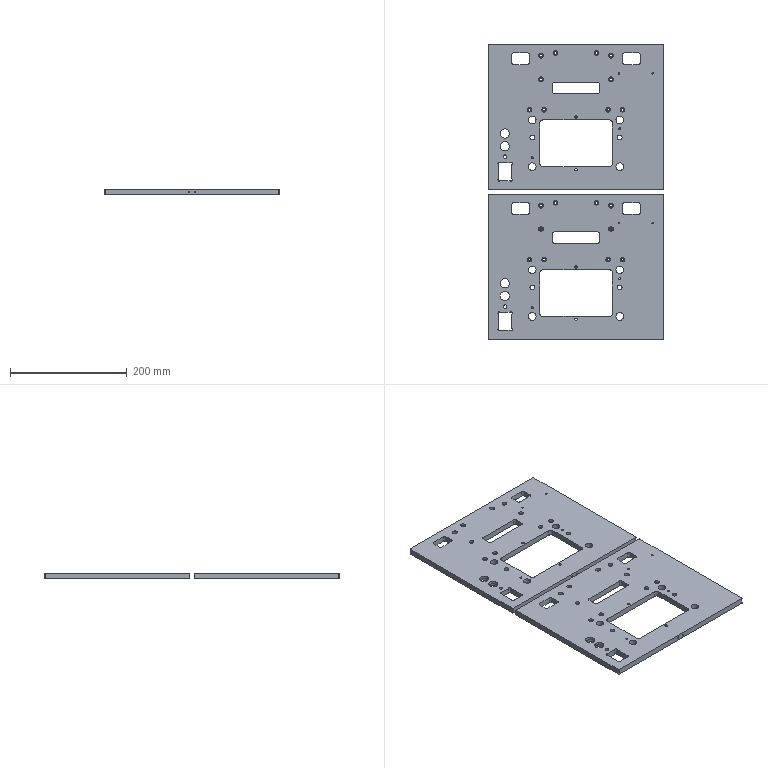NC program | NX | posted with a generic post | part box 300 x 507 x 10 mm
Whole program:
N10 G17 G21 G94 G90
(DRILLING_COPY , TOOL : D4A45)
N12 T02 M6
N14 G54
N16 G17 G0 G90 X122. Y-28. S5000 M3
N18 G43 Z30. H2
N20 G94 G81 G98 Z-1. F250. R3.
N22 Y-50.
N24 X121.5 Y-68.
N26 X131.7 Y-79.3
N28 Y-107.7
N30 X111.3
N32 Y-79.3
N34 X75. Y-85.
N36 Y-70.
N38 Y-35.
N40 Y-5.
N42 X80. Y12.5
N44 X54.75
N46 X54.8 Y44.8
N48 X65.2
N50 X60. Y65.
N52 Y105.
N54 X65.2 Y115.2
N56 X35. Y110.
N58 X-35.
N60 X-60. Y105.
N62 X-65.2 Y115.2
N64 X-131.5 Y75.
N66 X-73.5
N68 X-60. Y65.
N70 X-65.2 Y44.8
N72 X-54.8
N74 X-55.25 Y12.5
N76 X-80.
N78 X-75. Y-5.
N80 Y-20.
N82 Y-35.
N84 Y-85.
N86 X0. Y-90.
N88 Y0.
N90 G80
N92 G0 X0. Y0. Z30.
N94 M5
(HOLE_MILLING_COPY_COPY_COPY , TOOL : D6)
N96 T06 M6
N98 G54
N100 G17 G0 G90 X122. Y-28. S9500 M3
N102 G43 Z30. H6
N104 Z-4.5
N106 G94 G3 X120.75 Y-26.75 R1.25 F1500.
N108 X119.5 Y-28. R1.25
N110 X119.5 Y-28. Z-4.9 I2.5 J0.
N112 X119.5 Y-28. Z-5.3 I2.5 J0.
N114 X119.5 Y-28. Z-5.7 I2.5 J0.
N116 X119.5 Y-28. Z-6.1 I2.5 J0.
N118 X119.5 Y-28. Z-6.5 I2.5 J0.
N120 X119.5 Y-28. Z-6.9 I2.5 J0.
N122 X119.5 Y-28. Z-7.3 I2.5 J0.
N124 X119.5 Y-28. Z-7.7 I2.5 J0.
N126 X119.5 Y-28. Z-8.1 I2.5 J0.
N128 X119.5 Y-28. Z-8.5 I2.5 J0.
N130 X119.5 Y-28. Z-8.9 I2.5 J0.
N132 X119.5 Y-28. Z-9.3 I2.5 J0.
N134 X119.5 Y-28. Z-9.7 I2.5 J0.
N136 X122. Y-25.5 Z-10. R-2.5
N138 X119.5 Y-28. R2.5
N140 X122. Y-25.5 R-2.5
N142 X120.75 Y-26.75 R1.25
N144 X122. Y-28. R1.25
N146 G0 Z-4.5
N148 G3 X119.5 Y-25.5 R2.5
N150 X117. Y-28. R2.5
N152 X117. Y-28. Z-4.9 I5. J0.
N154 X117. Y-28. Z-5.3 I5. J0.
N156 X117. Y-28. Z-5.7 I5. J0.
N158 X117. Y-28. Z-6.1 I5. J0.
N160 X117. Y-28. Z-6.5 I5. J0.
N162 X117. Y-28. Z-6.9 I5. J0.
N164 X117. Y-28. Z-7.3 I5. J0.
N166 X117. Y-28. Z-7.7 I5. J0.
N168 X117. Y-28. Z-8.1 I5. J0.
N170 X117. Y-28. Z-8.5 I5. J0.
N172 X117. Y-28. Z-8.9 I5. J0.
N174 X117. Y-28. Z-9.3 I5. J0.
N176 X117. Y-28. Z-9.7 I5. J0.
N178 X122. Y-23. Z-10. R-5.
N180 X117. Y-28. R5.
N182 X122. Y-23. R-5.
N184 X119.5 Y-25.5 R2.5
N186 X122. Y-28. R2.5
N188 G0 Z30.
N190 Y-50.
N192 Z-4.5
N194 G3 X120.75 Y-48.75 R1.25
N196 X119.5 Y-50. R1.25
N198 X119.5 Y-50. Z-4.9 I2.5 J0.
N200 X119.5 Y-50. Z-5.3 I2.5 J0.
N202 X119.5 Y-50. Z-5.7 I2.5 J0.
N204 X119.5 Y-50. Z-6.1 I2.5 J0.
N206 X119.5 Y-50. Z-6.5 I2.5 J0.
N208 X119.5 Y-50. Z-6.9 I2.5 J0.
N210 X119.5 Y-50. Z-7.3 I2.5 J0.
N212 X119.5 Y-50. Z-7.7 I2.5 J0.
N214 X119.5 Y-50. Z-8.1 I2.5 J0.
N216 X119.5 Y-50. Z-8.5 I2.5 J0.
N218 X119.5 Y-50. Z-8.9 I2.5 J0.
N220 X119.5 Y-50. Z-9.3 I2.5 J0.
N222 X119.5 Y-50. Z-9.7 I2.5 J0.
N224 X122. Y-47.5 Z-10. R-2.5
N226 X119.5 Y-50. R2.5
N228 X122. Y-47.5 R-2.5
N230 X120.75 Y-48.75 R1.25
N232 X122. Y-50. R1.25
N234 G0 Z-4.5
N236 G3 X119.5 Y-47.5 R2.5
N238 X117. Y-50. R2.5
N240 X117. Y-50. Z-4.9 I5. J0.
N242 X117. Y-50. Z-5.3 I5. J0.
N244 X117. Y-50. Z-5.7 I5. J0.
N246 X117. Y-50. Z-6.1 I5. J0.
N248 X117. Y-50. Z-6.5 I5. J0.
N250 X117. Y-50. Z-6.9 I5. J0.
N252 X117. Y-50. Z-7.3 I5. J0.
N254 X117. Y-50. Z-7.7 I5. J0.
N256 X117. Y-50. Z-8.1 I5. J0.
N258 X117. Y-50. Z-8.5 I5. J0.
N260 X117. Y-50. Z-8.9 I5. J0.
N262 X117. Y-50. Z-9.3 I5. J0.
N264 X117. Y-50. Z-9.7 I5. J0.
N266 X122. Y-45. Z-10. R-5.
N268 X117. Y-50. R5.
N270 X122. Y-45. R-5.
N272 X119.5 Y-47.5 R2.5
N274 X122. Y-50. R2.5
N276 G0 Z30.
N278 M5
(ZLEVEL_PROFILE_COPY_COPY_COPY_COPY_COPY_COPY , TOOL : D4)
N280 T04 M6
N282 G54
N284 G17 G0 G90 X130.733 Y-106.436 S9500 M3
N286 G43 Z30. H4
N288 Z-8.5
N290 G94 G1 Z-10. F1000.
N292 X130.8 Y-106.397
N294 G3 X131. Y-106.051 R0.4
N296 G1 Y-80.949 F1200.
N298 G2 X131.762 Y-79.379 R2.
N300 G3 X131.621 Y-79.238 R-0.1
N302 G2 X130.051 Y-80. R2.
N304 G1 X112.949
N306 G2 X111.379 Y-79.238 R2.
N308 G1 X111.363 Y-79.222
N310 G3 X111.238 Y-79.379 R-0.1
N312 G2 X112. Y-80.949 R2.
N314 G1 Y-106.051
N316 G2 X111.238 Y-107.621 R2.
N318 G3 X111.275 Y-107.797 R0.1
N320 G1 X111.354 Y-107.793
N322 G2 X112.949 Y-107. R2.
N324 G1 X130.051
N326 G2 X131.621 Y-107.762 R2.
N328 G1 X131.634 Y-107.775
N330 X131.646 Y-107.793
N332 X131.723 Y-107.789
N334 X131.739 Y-107.792
N336 G3 X131.762 Y-107.621 R0.1
N338 G2 X131. Y-106.051 R2.
N340 G3 X130.8 Y-105.704 R0.4
N342 G1 X130.7 Y-105.647
N344 Z-8.5
N346 G0 Z30.
N348 X121.85 Y-68.606
N350 Z-8.5
N352 G1 Z-10. F1000.
N354 X122.3 Y-68.346
N356 G3 X122.5 Y-68. R0.4
N358 X121.5 Y-67. R1. F1200.
N360 X122.5 Y-68. R-1.
N362 X122.3 Y-67.654 R0.4
N364 G1 X121.85 Y-67.394
N366 Z-8.5
N368 G0 Z30.
N370 X127.685 Y-50.413
N372 Z-8.5
N374 G1 Z-10. F1000.
N376 X127.8 Y-50.346
N378 G3 X128. Y-50. R0.4
N380 X122. Y-44. R6. F1200.
N382 X128. Y-50. R-6.
N384 X127.8 Y-49.654 R0.4
N386 G1 X127.685 Y-49.587
N388 Z-8.5
N390 G0 Z30.
N392 Y-28.413
N394 Z-8.5
N396 G1 Z-10. F1000.
N398 X127.8 Y-28.346
N400 G3 X128. Y-28. R0.4
N402 X122. Y-22. R6. F1200.
N404 X128. Y-28. R-6.
N406 X127.8 Y-27.654 R0.4
N408 G1 X127.685 Y-27.587
N410 Z-8.5
N412 G0 Z30.
N414 X76.37 Y-88.97
N416 Z-8.5
N418 G1 Z-10. F1000.
N420 X76.485 Y-89.051
N422 G3 X76.883 Y-89.087 R0.4
N424 G1 X76.893 Y-89.082 F1200.
N426 G3 X71.48 Y-87.804 R-4.5
N428 G1 X71.612 Y-87.961
N430 G3 X76.883 Y-89.087 R4.5
N432 X77.114 Y-88.761 R0.4
N434 G1 X77.127 Y-88.622
N436 Z-8.5
N438 G0 Z30.
N440 X75.681 Y-36.558
N442 Z-8.5
N444 G1 Z-10. F1000.
N446 X75.856 Y-36.624
N448 G3 X76.251 Y-36.56 R0.4
N450 G1 X76.277 Y-36.539 F1200.
N452 G3 X73.723 Y-36.539 R-2.
N454 G1 X73.749 Y-36.56
N456 G3 X76.251 Y-36.56 R2.
N458 X76.396 Y-36.188 R0.4
N460 G1 X76.369 Y-36.008
N462 Z-8.5
N464 G0 Z30.
N466 X76.37 Y-8.97
N468 Z-8.5
N470 G1 Z-10. F1000.
N472 X76.485 Y-9.051
N474 G3 X76.883 Y-9.087 R0.4
N476 G1 X76.893 Y-9.082 F1200.
N478 G3 X71.48 Y-7.804 R-4.5
N480 G1 X71.612 Y-7.961
N482 G3 X76.883 Y-9.087 R4.5
N484 X77.114 Y-8.761 R0.4
N486 G1 X77.127 Y-8.622
N488 Z-8.5
N490 G0 Z30.
N492 X-78.753 Y-6.885
N494 Z-8.5
N496 G1 Z-10. F1000.
N498 X-78.818 Y-7.009
N500 G3 X-78.801 Y-7.408 R0.4
N502 G1 X-78.798 Y-7.414 F1200.
N504 G3 X-78.52 Y-7.804 R4.5
N506 G1 X-78.388 Y-7.961
N508 G3 X-78.801 Y-7.408 R-4.5
N510 X-78.447 Y-7.594 R0.4
N512 G1 X-78.308 Y-7.588
N514 Z-8.5
N516 G0 Z30.
N518 X-75.687 Y-33.445
N520 Z-8.5
N522 G1 Z-10. F1000.
N524 X-75.856 Y-33.379
N526 G3 X-76.251 Y-33.44 R0.4
N528 G1 X-76.257 Y-33.444 F1200.
N530 G3 X-76.277 Y-36.539 R2.
N532 G1 X-76.251 Y-36.56
N534 G3 X-73.749 Y-36.56 R2.
N536 G1 X-73.723 Y-36.539
N538 G3 X-76.251 Y-33.44 R2.
N540 X-76.396 Y-33.812 R0.4
N542 G1 X-76.369 Y-33.992
N544 Z-8.5
N546 G0 Z30.
N548 X-78.753 Y-86.885
N550 Z-8.5
N552 G1 Z-10. F1000.
N554 X-78.818 Y-87.009
N556 G3 X-78.801 Y-87.408 R0.4
N558 G1 X-78.798 Y-87.414 F1200.
N560 G3 X-78.52 Y-87.804 R4.5
N562 G1 X-78.388 Y-87.961
N564 G3 X-78.801 Y-87.408 R-4.5
N566 X-78.447 Y-87.594 R0.4
N568 G1 X-78.308 Y-87.588
N570 Z-8.5
N572 G0 Z30.
N574 M5
(CAVITY_MILL_COPY_COPY , TOOL : D3)
N576 T03 M6
N578 G54
N580 G17 G0 G90 X-62.028 Y113.1 S9500 M3
N582 G43 Z30. H3
N584 Z-0.2
N586 G94 G1 X-62.086 Y113.2 F1000.
N588 G3 X-62.952 Y113.7 R1.
N590 G1 X-63.7 F1200.
N592 Y112.952
N594 G3 X-63.2 Y112.086 R1.
N596 G1 X-63.1 Y112.028
N598 G0 X-62.028 Y113.1 Z-0.4
N600 G1 X-62.086 Y113.2 F1000.
N602 G3 X-62.952 Y113.7 R1.
N604 G1 X-63.7 F1200.
N606 Y112.952
N608 G3 X-63.2 Y112.086 R1.
N610 G1 X-63.1 Y112.028
N612 G0 X-62.028 Y113.1 Z-0.6
N614 G1 X-62.086 Y113.2 F1000.
N616 G3 X-62.952 Y113.7 R1.
N618 G1 X-63.7 F1200.
N620 Y112.952
N622 G3 X-63.2 Y112.086 R1.
N624 G1 X-63.1 Y112.028
N626 G0 X-62.028 Y113.1 Z-0.8
N628 G1 X-62.086 Y113.2 F1000.
N630 G3 X-62.952 Y113.7 R1.
N632 G1 X-63.7 F1200.
N634 Y112.952
N636 G3 X-63.2 Y112.086 R1.
N638 G1 X-63.1 Y112.028
N640 G0 X-62.028 Y113.1 Z-1.
N642 G1 X-62.086 Y113.2 F1000.
N644 G3 X-62.952 Y113.7 R1.
N646 G1 X-63.7 F1200.
N648 Y112.952
N650 G3 X-63.2 Y112.086 R1.
N652 G1 X-63.1 Y112.028
N654 G0 Z30.
N656 Y47.972
N658 Z-0.2
N660 G1 X-63.2 Y47.914 F1000.
N662 G3 X-63.7 Y47.048 R1.
N664 G1 Y46.3 F1200.
N666 X-62.952
N668 G3 X-62.086 Y46.8 R1.
N670 G1 X-62.028 Y46.9
N672 G0 X-63.1 Y47.972 Z-0.4
N674 G1 X-63.2 Y47.914 F1000.
N676 G3 X-63.7 Y47.048 R1.
N678 G1 Y46.3 F1200.
N680 X-62.952
N682 G3 X-62.086 Y46.8 R1.
N684 G1 X-62.028 Y46.9
N686 G0 X-63.1 Y47.972 Z-0.6
N688 G1 X-63.2 Y47.914 F1000.
N690 G3 X-63.7 Y47.048 R1.
N692 G1 Y46.3 F1200.
N694 X-62.952
N696 G3 X-62.086 Y46.8 R1.
N698 G1 X-62.028 Y46.9
N700 G0 X-63.1 Y47.972 Z-0.8
N702 G1 X-63.2 Y47.914 F1000.
N704 G3 X-63.7 Y47.048 R1.
N706 G1 Y46.3 F1200.
N708 X-62.952
N710 G3 X-62.086 Y46.8 R1.
N712 G1 X-62.028 Y46.9
N714 G0 X-63.1 Y47.972 Z-1.
N716 G1 X-63.2 Y47.914 F1000.
N718 G3 X-63.7 Y47.048 R1.
N720 G1 Y46.3 F1200.
N722 X-62.952
N724 G3 X-62.086 Y46.8 R1.
N726 G1 X-62.028 Y46.9
N728 G0 Z30.
N730 X-57.972
N732 Z-0.2
N734 G1 X-57.914 Y46.8 F1000.
N736 G3 X-57.048 Y46.3 R1.
N738 G1 X-56.3 F1200.
N740 Y47.048
N742 G3 X-56.8 Y47.914 R1.
N744 G1 X-56.9 Y47.972
N746 G0 X-57.972 Y46.9 Z-0.4
N748 G1 X-57.914 Y46.8 F1000.
N750 G3 X-57.048 Y46.3 R1.
N752 G1 X-56.3 F1200.
N754 Y47.048
N756 G3 X-56.8 Y47.914 R1.
N758 G1 X-56.9 Y47.972
N760 G0 X-57.972 Y46.9 Z-0.6
N762 G1 X-57.914 Y46.8 F1000.
N764 G3 X-57.048 Y46.3 R1.
N766 G1 X-56.3 F1200.
N768 Y47.048
N770 G3 X-56.8 Y47.914 R1.
N772 G1 X-56.9 Y47.972
N774 G0 X-57.972 Y46.9 Z-0.8
N776 G1 X-57.914 Y46.8 F1000.
N778 G3 X-57.048 Y46.3 R1.
N780 G1 X-56.3 F1200.
N782 Y47.048
N784 G3 X-56.8 Y47.914 R1.
N786 G1 X-56.9 Y47.972
N788 G0 X-57.972 Y46.9 Z-1.
N790 G1 X-57.914 Y46.8 F1000.
N792 G3 X-57.048 Y46.3 R1.
N794 G1 X-56.3 F1200.
N796 Y47.048
N798 G3 X-56.8 Y47.914 R1.
N800 G1 X-56.9 Y47.972
N802 G0 Z30.
N804 X56.9
N806 Z-0.2
N808 G1 X56.8 Y47.914 F1000.
N810 G3 X56.3 Y47.048 R1.
N812 G1 Y46.3 F1200.
N814 X57.048
N816 G3 X57.914 Y46.8 R1.
N818 G1 X57.972 Y46.9
N820 G0 X56.9 Y47.972 Z-0.4
N822 G1 X56.8 Y47.914 F1000.
N824 G3 X56.3 Y47.048 R1.
N826 G1 Y46.3 F1200.
N828 X57.048
N830 G3 X57.914 Y46.8 R1.
N832 G1 X57.972 Y46.9
N834 G0 X56.9 Y47.972 Z-0.6
N836 G1 X56.8 Y47.914 F1000.
N838 G3 X56.3 Y47.048 R1.
N840 G1 Y46.3 F1200.
N842 X57.048
N844 G3 X57.914 Y46.8 R1.
N846 G1 X57.972 Y46.9
N848 G0 X56.9 Y47.972 Z-0.8
N850 G1 X56.8 Y47.914 F1000.
N852 G3 X56.3 Y47.048 R1.
N854 G1 Y46.3 F1200.
N856 X57.048
N858 G3 X57.914 Y46.8 R1.
N860 G1 X57.972 Y46.9
N862 G0 X56.9 Y47.972 Z-1.
N864 G1 X56.8 Y47.914 F1000.
N866 G3 X56.3 Y47.048 R1.
N868 G1 Y46.3 F1200.
N870 X57.048
N872 G3 X57.914 Y46.8 R1.
N874 G1 X57.972 Y46.9
N876 G0 Z30.
N878 X62.028
N880 Z-0.2
N882 G1 X62.086 Y46.8 F1000.
N884 G3 X62.952 Y46.3 R1.
N886 G1 X63.7 F1200.
N888 Y47.048
N890 G3 X63.2 Y47.914 R1.
N892 G1 X63.1 Y47.972
N894 G0 X62.028 Y46.9 Z-0.4
N896 G1 X62.086 Y46.8 F1000.
N898 G3 X62.952 Y46.3 R1.
N900 G1 X63.7 F1200.
N902 Y47.048
N904 G3 X63.2 Y47.914 R1.
N906 G1 X63.1 Y47.972
N908 G0 X62.028 Y46.9 Z-0.6
N910 G1 X62.086 Y46.8 F1000.
N912 G3 X62.952 Y46.3 R1.
N914 G1 X63.7 F1200.
N916 Y47.048
N918 G3 X63.2 Y47.914 R1.
N920 G1 X63.1 Y47.972
N922 G0 X62.028 Y46.9 Z-0.8
N924 G1 X62.086 Y46.8 F1000.
N926 G3 X62.952 Y46.3 R1.
N928 G1 X63.7 F1200.
N930 Y47.048
N932 G3 X63.2 Y47.914 R1.
N934 G1 X63.1 Y47.972
N936 G0 X62.028 Y46.9 Z-1.
N938 G1 X62.086 Y46.8 F1000.
N940 G3 X62.952 Y46.3 R1.
N942 G1 X63.7 F1200.
N944 Y47.048
N946 G3 X63.2 Y47.914 R1.
N948 G1 X63.1 Y47.972
N950 G0 Z30.
N952 Y112.028
N954 Z-0.2
N956 G1 X63.2 Y112.086 F1000.
N958 G3 X63.7 Y112.952 R1.
N960 G1 Y113.7 F1200.
N962 X62.952
N964 G3 X62.086 Y113.2 R1.
N966 G1 X62.028 Y113.1
N968 G0 X63.1 Y112.028 Z-0.4
N970 G1 X63.2 Y112.086 F1000.
N972 G3 X63.7 Y112.952 R1.
N974 G1 Y113.7 F1200.
N976 X62.952
N978 G3 X62.086 Y113.2 R1.
N980 G1 X62.028 Y113.1
N982 G0 X63.1 Y112.028 Z-0.6
N984 G1 X63.2 Y112.086 F1000.
N986 G3 X63.7 Y112.952 R1.
N988 G1 Y113.7 F1200.
N990 X62.952
N992 G3 X62.086 Y113.2 R1.
N994 G1 X62.028 Y113.1
N996 G0 X63.1 Y112.028 Z-0.8
N998 G1 X63.2 Y112.086 F1000.
N1000 G3 X63.7 Y112.952 R1.
N1002 G1 Y113.7 F1200.
N1004 X62.952
N1006 G3 X62.086 Y113.2 R1.
N1008 G1 X62.028 Y113.1
N1010 G0 X63.1 Y112.028 Z-1.
N1012 G1 X63.2 Y112.086 F1000.
N1014 G3 X63.7 Y112.952 R1.
N1016 G1 Y113.7 F1200.
N1018 X62.952
N1020 G3 X62.086 Y113.2 R1.
N1022 G1 X62.028 Y113.1
N1024 G0 Z30.
N1026 M5
N1028 M2